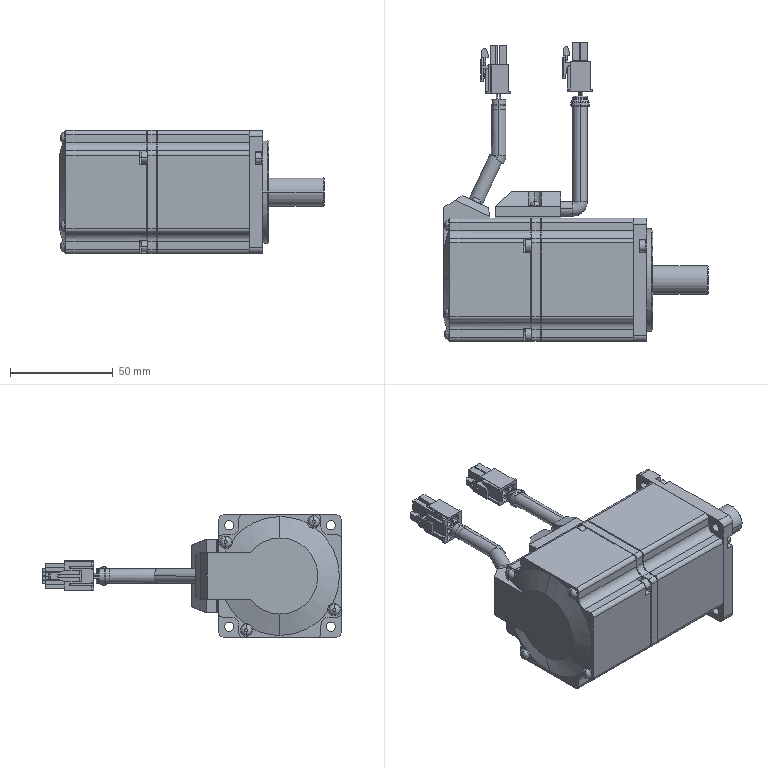Part | SolidWorks | features BaseBody 2 | 2 solids | 771 faces | box 129 x 145.8 x 60 mm | volume 348980 mm3 | plane 490 | cylinder 227 | cone 27 | spline 14 | torus 13 | commonest cylinder face diameters 4 x47 8 x24 2.6 x20 1 x18 4.5 x16 5.5 x16